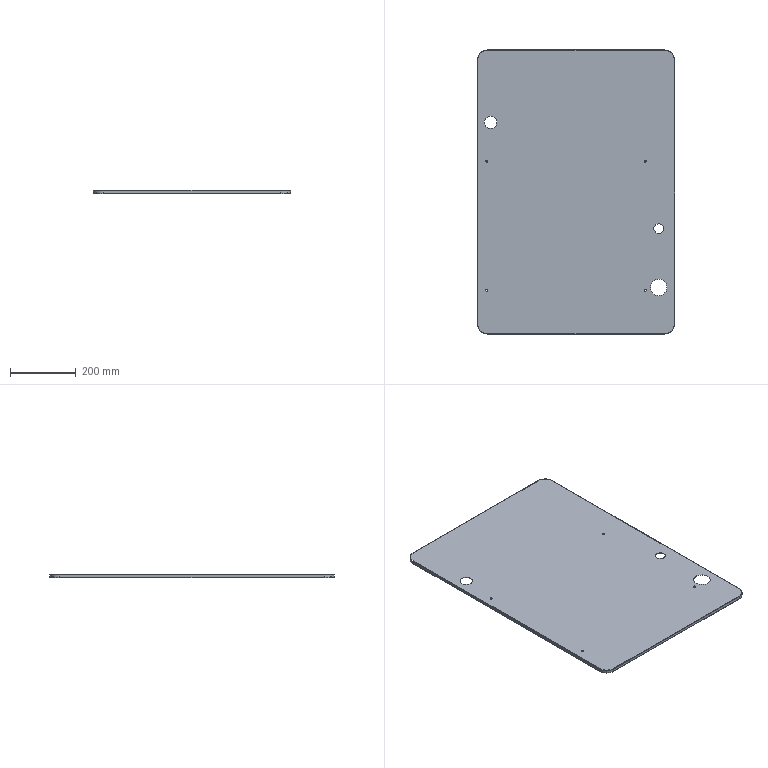Part | STEP file | HESS-408-70-15W-N-3-inner liner rear panel | 1 solid | 88 faces | box 600 x 864.78 x 10 mm | volume 539176 mm3 | plane 46 | cylinder 42 | commonest cylinder face diameters 6 x8 58 x8 60 x8 0.1 x4 2.1 x4 57.8 x4